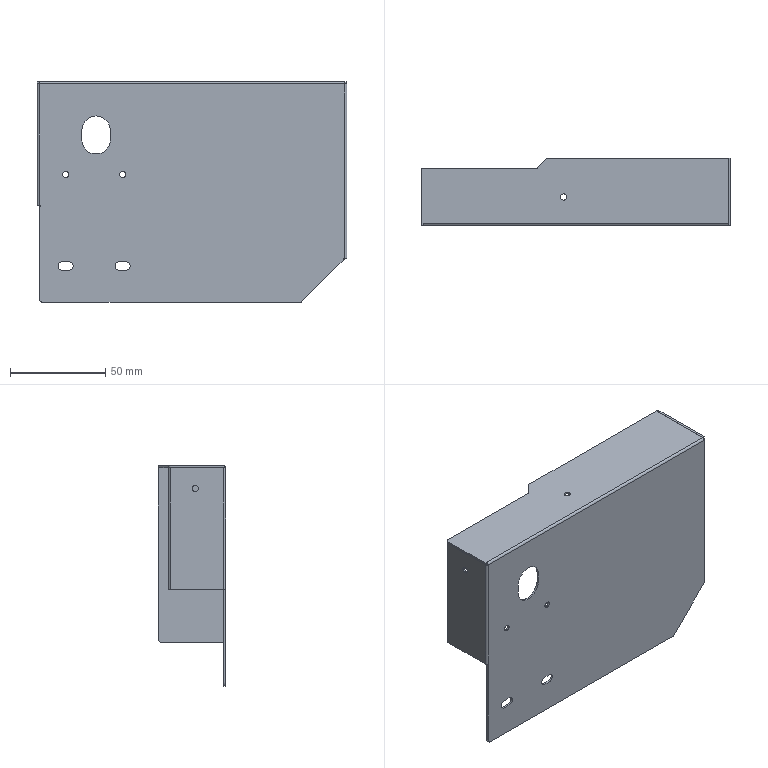Part | STEP file | motor fixing plate | 1 solid | 84 faces | box 163 x 35.5 x 116 mm | volume 28996 mm3 | plane 54 | cylinder 30 | commonest cylinder face diameters 3.3 x8 0.1 x4 2 x4 2.1 x4 4.5 x4 4 x3